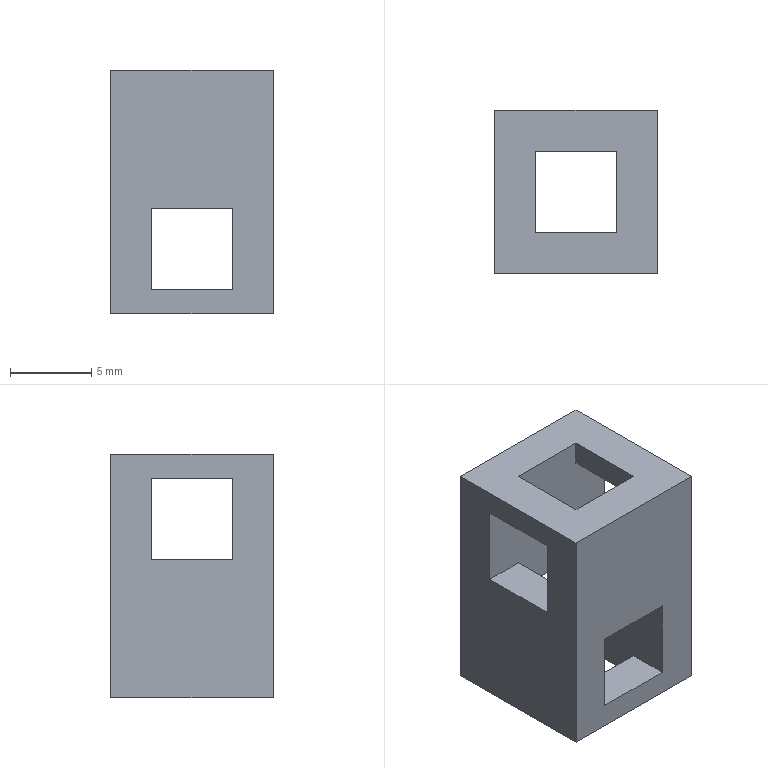Part | SolidWorks | features ICE 2, Extrusion 1 | 1 solid | 22 faces | box 10 x 10 x 15 mm | volume 875 mm3 | plane 22
STEP:
#1=CARTESIAN_POINT('',(2.5,2.5,8.5));
#2=VERTEX_POINT('',#1);
#3=CARTESIAN_POINT('',(2.5,-2.5,8.5));
#4=VERTEX_POINT('',#3);
#5=CARTESIAN_POINT('',(2.5,2.5,8.5));
#6=DIRECTION('',(0.,-1.,0.));
#7=VECTOR('',#6,1000.);
#8=LINE('',#5,#7);
#9=EDGE_CURVE('',#2,#4,#8,.T.);
#10=ORIENTED_EDGE('',*,*,#9,.F.);
#11=CARTESIAN_POINT('',(2.5,2.5,6.5));
#12=VERTEX_POINT('',#11);
#13=CARTESIAN_POINT('',(2.5,2.5,15.));
#14=DIRECTION('',(0.,0.,-1.));
#15=VECTOR('',#14,1000.);
#16=LINE('',#13,#15);
#17=EDGE_CURVE('',#2,#12,#16,.T.);
#18=ORIENTED_EDGE('',*,*,#17,.T.);
#19=CARTESIAN_POINT('',(2.5,5.,6.5));
#20=VERTEX_POINT('',#19);
#21=CARTESIAN_POINT('',(2.5,-5.,6.5));
#22=DIRECTION('',(0.,1.,0.));
#23=VECTOR('',#22,1000.);
#24=LINE('',#21,#23);
#25=EDGE_CURVE('',#12,#20,#24,.T.);
#26=ORIENTED_EDGE('',*,*,#25,.T.);
#27=CARTESIAN_POINT('',(2.5,5.,1.5));
#28=VERTEX_POINT('',#27);
#29=CARTESIAN_POINT('',(2.5,5.,1.5));
#30=DIRECTION('',(0.,0.,-1.));
#31=VECTOR('',#30,1000.);
#32=LINE('',#29,#31);
#33=EDGE_CURVE('',#20,#28,#32,.T.);
#34=ORIENTED_EDGE('',*,*,#33,.T.);
#35=CARTESIAN_POINT('',(2.5,2.5,1.5));
#36=VERTEX_POINT('',#35);
#37=CARTESIAN_POINT('',(2.5,-5.,1.5));
#38=DIRECTION('',(0.,1.,0.));
#39=VECTOR('',#38,1000.);
#40=LINE('',#37,#39);
#41=EDGE_CURVE('',#36,#28,#40,.T.);
#42=ORIENTED_EDGE('',*,*,#41,.F.);
#43=CARTESIAN_POINT('',(2.5,2.5,0.));
#44=VERTEX_POINT('',#43);
#45=CARTESIAN_POINT('',(2.5,2.5,15.));
#46=DIRECTION('',(0.,0.,-1.));
#47=VECTOR('',#46,1000.);
#48=LINE('',#45,#47);
#49=EDGE_CURVE('',#36,#44,#48,.T.);
#50=ORIENTED_EDGE('',*,*,#49,.T.);
#51=CARTESIAN_POINT('',(2.5,-2.5,0.));
#52=VERTEX_POINT('',#51);
#53=CARTESIAN_POINT('',(2.5,2.5,0.));
#54=DIRECTION('',(0.,1.,0.));
#55=VECTOR('',#54,1000.);
#56=LINE('',#53,#55);
#57=EDGE_CURVE('',#52,#44,#56,.T.);
#58=ORIENTED_EDGE('',*,*,#57,.F.);
#59=CARTESIAN_POINT('',(2.5,-2.5,1.5));
#60=VERTEX_POINT('',#59);
#61=CARTESIAN_POINT('',(2.5,-2.5,15.));
#62=DIRECTION('',(0.,0.,-1.));
#63=VECTOR('',#62,1000.);
#64=LINE('',#61,#63);
#65=EDGE_CURVE('',#60,#52,#64,.T.);
#66=ORIENTED_EDGE('',*,*,#65,.F.);
#67=CARTESIAN_POINT('',(2.5,-5.,1.5));
#68=VERTEX_POINT('',#67);
#69=CARTESIAN_POINT('',(2.5,-5.,1.5));
#70=DIRECTION('',(0.,1.,0.));
#71=VECTOR('',#70,1000.);
#72=LINE('',#69,#71);
#73=EDGE_CURVE('',#68,#60,#72,.T.);
#74=ORIENTED_EDGE('',*,*,#73,.F.);
#75=CARTESIAN_POINT('',(2.5,-5.,6.5));
#76=VERTEX_POINT('',#75);
#77=CARTESIAN_POINT('',(2.5,-5.,1.5));
#78=DIRECTION('',(0.,0.,-1.));
#79=VECTOR('',#78,1000.);
#80=LINE('',#77,#79);
#81=EDGE_CURVE('',#76,#68,#80,.T.);
#82=ORIENTED_EDGE('',*,*,#81,.F.);
#83=CARTESIAN_POINT('',(2.5,-2.5,6.5));
#84=VERTEX_POINT('',#83);
#85=CARTESIAN_POINT('',(2.5,-5.,6.5));
#86=DIRECTION('',(0.,1.,0.));
#87=VECTOR('',#86,1000.);
#88=LINE('',#85,#87);
#89=EDGE_CURVE('',#76,#84,#88,.T.);
#90=ORIENTED_EDGE('',*,*,#89,.T.);
#91=CARTESIAN_POINT('',(2.5,-2.5,15.));
#92=DIRECTION('',(0.,0.,-1.));
#93=VECTOR('',#92,1000.);
#94=LINE('',#91,#93);
#95=EDGE_CURVE('',#4,#84,#94,.T.);
#96=ORIENTED_EDGE('',*,*,#95,.F.);
#97=EDGE_LOOP('',(#10,#18,#26,#34,#42,#50,#58,#66,#74,#82,#90,#96));
#98=FACE_OUTER_BOUND('',#97,.T.);
#99=CARTESIAN_POINT('',(2.5,2.5,15.));
#100=DIRECTION('',(-1.,0.,0.));
#101=DIRECTION('',(0.,-1.,0.));
#102=AXIS2_PLACEMENT_3D('',#99,#100,#101);
#103=PLANE('',#102);
#104=ADVANCED_FACE('',(#98),#103,.T.);
#105=CARTESIAN_POINT('',(-2.5,-2.5,8.5));
#106=VERTEX_POINT('',#105);
#107=CARTESIAN_POINT('',(-2.5,2.5,8.5));
#108=VERTEX_POINT('',#107);
#109=CARTESIAN_POINT('',(-2.5,2.5,8.5));
#110=DIRECTION('',(0.,1.,0.));
#111=VECTOR('',#110,1000.);
#112=LINE('',#109,#111);
#113=EDGE_CURVE('',#106,#108,#112,.T.);
#114=ORIENTED_EDGE('',*,*,#113,.F.);
#115=CARTESIAN_POINT('',(-2.5,-2.5,6.5));
#116=VERTEX_POINT('',#115);
#117=CARTESIAN_POINT('',(-2.5,-2.5,15.));
#118=DIRECTION('',(0.,0.,-1.));
#119=VECTOR('',#118,1000.);
#120=LINE('',#117,#119);
#121=EDGE_CURVE('',#106,#116,#120,.T.);
#122=ORIENTED_EDGE('',*,*,#121,.T.);
#123=CARTESIAN_POINT('',(-2.5,-5.,6.5));
#124=VERTEX_POINT('',#123);
#125=CARTESIAN_POINT('',(-2.5,-5.,6.5));
#126=DIRECTION('',(0.,1.,0.));
#127=VECTOR('',#126,1000.);
#128=LINE('',#125,#127);
#129=EDGE_CURVE('',#124,#116,#128,.T.);
#130=ORIENTED_EDGE('',*,*,#129,.F.);
#131=CARTESIAN_POINT('',(-2.5,-5.,1.5));
#132=VERTEX_POINT('',#131);
#133=CARTESIAN_POINT('',(-2.5,-5.,1.5));
#134=DIRECTION('',(0.,0.,1.));
#135=VECTOR('',#134,1000.);
#136=LINE('',#133,#135);
#137=EDGE_CURVE('',#132,#124,#136,.T.);
#138=ORIENTED_EDGE('',*,*,#137,.F.);
#139=CARTESIAN_POINT('',(-2.5,-2.5,1.5));
#140=VERTEX_POINT('',#139);
#141=CARTESIAN_POINT('',(-2.5,-5.,1.5));
#142=DIRECTION('',(0.,1.,0.));
#143=VECTOR('',#142,1000.);
#144=LINE('',#141,#143);
#145=EDGE_CURVE('',#132,#140,#144,.T.);
#146=ORIENTED_EDGE('',*,*,#145,.T.);
#147=CARTESIAN_POINT('',(-2.5,-2.5,0.));
#148=VERTEX_POINT('',#147);
#149=CARTESIAN_POINT('',(-2.5,-2.5,15.));
#150=DIRECTION('',(0.,0.,-1.));
#151=VECTOR('',#150,1000.);
#152=LINE('',#149,#151);
#153=EDGE_CURVE('',#140,#148,#152,.T.);
#154=ORIENTED_EDGE('',*,*,#153,.T.);
#155=CARTESIAN_POINT('',(-2.5,2.5,0.));
#156=VERTEX_POINT('',#155);
#157=CARTESIAN_POINT('',(-2.5,2.5,0.));
#158=DIRECTION('',(0.,-1.,0.));
#159=VECTOR('',#158,1000.);
#160=LINE('',#157,#159);
#161=EDGE_CURVE('',#156,#148,#160,.T.);
#162=ORIENTED_EDGE('',*,*,#161,.F.);
#163=CARTESIAN_POINT('',(-2.5,2.5,1.5));
#164=VERTEX_POINT('',#163);
#165=CARTESIAN_POINT('',(-2.5,2.5,15.));
#166=DIRECTION('',(0.,0.,-1.));
#167=VECTOR('',#166,1000.);
#168=LINE('',#165,#167);
#169=EDGE_CURVE('',#164,#156,#168,.T.);
#170=ORIENTED_EDGE('',*,*,#169,.F.);
#171=CARTESIAN_POINT('',(-2.5,5.,1.5));
#172=VERTEX_POINT('',#171);
#173=CARTESIAN_POINT('',(-2.5,-5.,1.5));
#174=DIRECTION('',(0.,1.,0.));
#175=VECTOR('',#174,1000.);
#176=LINE('',#173,#175);
#177=EDGE_CURVE('',#164,#172,#176,.T.);
#178=ORIENTED_EDGE('',*,*,#177,.T.);
#179=CARTESIAN_POINT('',(-2.5,5.,6.5));
#180=VERTEX_POINT('',#179);
#181=CARTESIAN_POINT('',(-2.5,5.,1.5));
#182=DIRECTION('',(0.,0.,1.));
#183=VECTOR('',#182,1000.);
#184=LINE('',#181,#183);
#185=EDGE_CURVE('',#172,#180,#184,.T.);
#186=ORIENTED_EDGE('',*,*,#185,.T.);
#187=CARTESIAN_POINT('',(-2.5,2.5,6.5));
#188=VERTEX_POINT('',#187);
#189=CARTESIAN_POINT('',(-2.5,-5.,6.5));
#190=DIRECTION('',(0.,1.,0.));
#191=VECTOR('',#190,1000.);
#192=LINE('',#189,#191);
#193=EDGE_CURVE('',#188,#180,#192,.T.);
#194=ORIENTED_EDGE('',*,*,#193,.F.);
#195=CARTESIAN_POINT('',(-2.5,2.5,15.));
#196=DIRECTION('',(0.,0.,-1.));
#197=VECTOR('',#196,1000.);
#198=LINE('',#195,#197);
#199=EDGE_CURVE('',#108,#188,#198,.T.);
#200=ORIENTED_EDGE('',*,*,#199,.F.);
#201=EDGE_LOOP('',(#114,#122,#130,#138,#146,#154,#162,#170,#178,#186,#194,#200));
#202=FACE_OUTER_BOUND('',#201,.T.);
#203=CARTESIAN_POINT('',(-2.5,2.5,15.));
#204=DIRECTION('',(1.,0.,0.));
#205=DIRECTION('',(0.,1.,0.));
#206=AXIS2_PLACEMENT_3D('',#203,#204,#205);
#207=PLANE('',#206);
#208=ADVANCED_FACE('',(#202),#207,.T.);
#209=CARTESIAN_POINT('',(-2.5,2.5,15.));
#210=VERTEX_POINT('',#209);
#211=CARTESIAN_POINT('',(-2.5,2.5,13.5));
#212=VERTEX_POINT('',#211);
#213=CARTESIAN_POINT('',(-2.5,2.5,15.));
#214=DIRECTION('',(0.,0.,-1.));
#215=VECTOR('',#214,1000.);
#216=LINE('',#213,#215);
#217=EDGE_CURVE('',#210,#212,#216,.T.);
#218=ORIENTED_EDGE('',*,*,#217,.T.);
#219=CARTESIAN_POINT('',(-5.,2.5,13.5));
#220=VERTEX_POINT('',#219);
#221=CARTESIAN_POINT('',(-5.,2.5,13.5));
#222=DIRECTION('',(1.,0.,0.));
#223=VECTOR('',#222,1000.);
#224=LINE('',#221,#223);
#225=EDGE_CURVE('',#220,#212,#224,.T.);
#226=ORIENTED_EDGE('',*,*,#225,.F.);
#227=CARTESIAN_POINT('',(-5.,2.5,8.5));
#228=VERTEX_POINT('',#227);
#229=CARTESIAN_POINT('',(-5.,2.5,13.5));
#230=DIRECTION('',(0.,0.,1.));
#231=VECTOR('',#230,1000.);
#232=LINE('',#229,#231);
#233=EDGE_CURVE('',#228,#220,#232,.T.);
#234=ORIENTED_EDGE('',*,*,#233,.F.);
#235=CARTESIAN_POINT('',(-5.,2.5,8.5));
#236=DIRECTION('',(1.,0.,0.));
#237=VECTOR('',#236,1000.);
#238=LINE('',#235,#237);
#239=EDGE_CURVE('',#228,#108,#238,.T.);
#240=ORIENTED_EDGE('',*,*,#239,.T.);
#241=ORIENTED_EDGE('',*,*,#199,.T.);
#242=CARTESIAN_POINT('',(-2.5,2.5,6.5));
#243=DIRECTION('',(-1.,0.,0.));
#244=VECTOR('',#243,1000.);
#245=LINE('',#242,#244);
#246=EDGE_CURVE('',#12,#188,#245,.T.);
#247=ORIENTED_EDGE('',*,*,#246,.F.);
#248=ORIENTED_EDGE('',*,*,#17,.F.);
#249=CARTESIAN_POINT('',(5.,2.5,8.5));
#250=VERTEX_POINT('',#249);
#251=CARTESIAN_POINT('',(-5.,2.5,8.5));
#252=DIRECTION('',(1.,0.,0.));
#253=VECTOR('',#252,1000.);
#254=LINE('',#251,#253);
#255=EDGE_CURVE('',#2,#250,#254,.T.);
#256=ORIENTED_EDGE('',*,*,#255,.T.);
#257=CARTESIAN_POINT('',(5.,2.5,13.5));
#258=VERTEX_POINT('',#257);
#259=CARTESIAN_POINT('',(5.,2.5,13.5));
#260=DIRECTION('',(0.,0.,1.));
#261=VECTOR('',#260,1000.);
#262=LINE('',#259,#261);
#263=EDGE_CURVE('',#250,#258,#262,.T.);
#264=ORIENTED_EDGE('',*,*,#263,.T.);
#265=CARTESIAN_POINT('',(2.5,2.5,13.5));
#266=VERTEX_POINT('',#265);
#267=CARTESIAN_POINT('',(-5.,2.5,13.5));
#268=DIRECTION('',(1.,0.,0.));
#269=VECTOR('',#268,1000.);
#270=LINE('',#267,#269);
#271=EDGE_CURVE('',#266,#258,#270,.T.);
#272=ORIENTED_EDGE('',*,*,#271,.F.);
#273=CARTESIAN_POINT('',(2.5,2.5,15.));
#274=VERTEX_POINT('',#273);
#275=CARTESIAN_POINT('',(2.5,2.5,15.));
#276=DIRECTION('',(0.,0.,-1.));
#277=VECTOR('',#276,1000.);
#278=LINE('',#275,#277);
#279=EDGE_CURVE('',#274,#266,#278,.T.);
#280=ORIENTED_EDGE('',*,*,#279,.F.);
#281=CARTESIAN_POINT('',(-2.5,2.5,15.));
#282=DIRECTION('',(-1.,0.,0.));
#283=VECTOR('',#282,1000.);
#284=LINE('',#281,#283);
#285=EDGE_CURVE('',#274,#210,#284,.T.);
#286=ORIENTED_EDGE('',*,*,#285,.T.);
#287=EDGE_LOOP('',(#218,#226,#234,#240,#241,#247,#248,#256,#264,#272,#280,#286));
#288=FACE_OUTER_BOUND('',#287,.T.);
#289=CARTESIAN_POINT('',(-2.5,2.5,15.));
#290=DIRECTION('',(0.,-1.,0.));
#291=DIRECTION('',(0.,0.,-1.));
#292=AXIS2_PLACEMENT_3D('',#289,#290,#291);
#293=PLANE('',#292);
#294=ADVANCED_FACE('',(#288),#293,.T.);
#295=CARTESIAN_POINT('',(2.5,-2.5,15.));
#296=VERTEX_POINT('',#295);
#297=CARTESIAN_POINT('',(2.5,-2.5,13.5));
#298=VERTEX_POINT('',#297);
#299=CARTESIAN_POINT('',(2.5,-2.5,15.));
#300=DIRECTION('',(0.,0.,-1.));
#301=VECTOR('',#300,1000.);
#302=LINE('',#299,#301);
#303=EDGE_CURVE('',#296,#298,#302,.T.);
#304=ORIENTED_EDGE('',*,*,#303,.T.);
#305=CARTESIAN_POINT('',(5.,-2.5,13.5));
#306=VERTEX_POINT('',#305);
#307=CARTESIAN_POINT('',(-5.,-2.5,13.5));
#308=DIRECTION('',(1.,0.,0.));
#309=VECTOR('',#308,1000.);
#310=LINE('',#307,#309);
#311=EDGE_CURVE('',#298,#306,#310,.T.);
#312=ORIENTED_EDGE('',*,*,#311,.T.);
#313=CARTESIAN_POINT('',(5.,-2.5,8.5));
#314=VERTEX_POINT('',#313);
#315=CARTESIAN_POINT('',(5.,-2.5,13.5));
#316=DIRECTION('',(0.,0.,-1.));
#317=VECTOR('',#316,1000.);
#318=LINE('',#315,#317);
#319=EDGE_CURVE('',#306,#314,#318,.T.);
#320=ORIENTED_EDGE('',*,*,#319,.T.);
#321=CARTESIAN_POINT('',(-5.,-2.5,8.5));
#322=DIRECTION('',(1.,0.,0.));
#323=VECTOR('',#322,1000.);
#324=LINE('',#321,#323);
#325=EDGE_CURVE('',#4,#314,#324,.T.);
#326=ORIENTED_EDGE('',*,*,#325,.F.);
#327=ORIENTED_EDGE('',*,*,#95,.T.);
#328=CARTESIAN_POINT('',(-2.5,-2.5,6.5));
#329=DIRECTION('',(1.,0.,0.));
#330=VECTOR('',#329,1000.);
#331=LINE('',#328,#330);
#332=EDGE_CURVE('',#116,#84,#331,.T.);
#333=ORIENTED_EDGE('',*,*,#332,.F.);
#334=ORIENTED_EDGE('',*,*,#121,.F.);
#335=CARTESIAN_POINT('',(-5.,-2.5,8.5));
#336=VERTEX_POINT('',#335);
#337=CARTESIAN_POINT('',(-5.,-2.5,8.5));
#338=DIRECTION('',(1.,0.,0.));
#339=VECTOR('',#338,1000.);
#340=LINE('',#337,#339);
#341=EDGE_CURVE('',#336,#106,#340,.T.);
#342=ORIENTED_EDGE('',*,*,#341,.F.);
#343=CARTESIAN_POINT('',(-5.,-2.5,13.5));
#344=VERTEX_POINT('',#343);
#345=CARTESIAN_POINT('',(-5.,-2.5,13.5));
#346=DIRECTION('',(0.,0.,-1.));
#347=VECTOR('',#346,1000.);
#348=LINE('',#345,#347);
#349=EDGE_CURVE('',#344,#336,#348,.T.);
#350=ORIENTED_EDGE('',*,*,#349,.F.);
#351=CARTESIAN_POINT('',(-2.5,-2.5,13.5));
#352=VERTEX_POINT('',#351);
#353=CARTESIAN_POINT('',(-5.,-2.5,13.5));
#354=DIRECTION('',(1.,0.,0.));
#355=VECTOR('',#354,1000.);
#356=LINE('',#353,#355);
#357=EDGE_CURVE('',#344,#352,#356,.T.);
#358=ORIENTED_EDGE('',*,*,#357,.T.);
#359=CARTESIAN_POINT('',(-2.5,-2.5,15.));
#360=VERTEX_POINT('',#359);
#361=CARTESIAN_POINT('',(-2.5,-2.5,15.));
#362=DIRECTION('',(0.,0.,-1.));
#363=VECTOR('',#362,1000.);
#364=LINE('',#361,#363);
#365=EDGE_CURVE('',#360,#352,#364,.T.);
#366=ORIENTED_EDGE('',*,*,#365,.F.);
#367=CARTESIAN_POINT('',(-2.5,-2.5,15.));
#368=DIRECTION('',(1.,0.,0.));
#369=VECTOR('',#368,1000.);
#370=LINE('',#367,#369);
#371=EDGE_CURVE('',#360,#296,#370,.T.);
#372=ORIENTED_EDGE('',*,*,#371,.T.);
#373=EDGE_LOOP('',(#304,#312,#320,#326,#327,#333,#334,#342,#350,#358,#366,#372));
#374=FACE_OUTER_BOUND('',#373,.T.);
#375=CARTESIAN_POINT('',(-2.5,-2.5,15.));
#376=DIRECTION('',(0.,1.,0.));
#377=DIRECTION('',(0.,0.,1.));
#378=AXIS2_PLACEMENT_3D('',#375,#376,#377);
#379=PLANE('',#378);
#380=ADVANCED_FACE('',(#374),#379,.T.);
#381=CARTESIAN_POINT('',(5.,-5.,15.));
#382=VERTEX_POINT('',#381);
#383=CARTESIAN_POINT('',(5.,5.,15.));
#384=VERTEX_POINT('',#383);
#385=CARTESIAN_POINT('',(5.,5.,15.));
#386=DIRECTION('',(0.,1.,0.));
#387=VECTOR('',#386,1000.);
#388=LINE('',#385,#387);
#389=EDGE_CURVE('',#382,#384,#388,.T.);
#390=ORIENTED_EDGE('',*,*,#389,.T.);
#391=CARTESIAN_POINT('',(-5.,5.,15.));
#392=VERTEX_POINT('',#391);
#393=CARTESIAN_POINT('',(-5.,5.,15.));
#394=DIRECTION('',(-1.,0.,0.));
#395=VECTOR('',#394,1000.);
#396=LINE('',#393,#395);
#397=EDGE_CURVE('',#384,#392,#396,.T.);
#398=ORIENTED_EDGE('',*,*,#397,.T.);
#399=CARTESIAN_POINT('',(-5.,-5.,15.));
#400=VERTEX_POINT('',#399);
#401=CARTESIAN_POINT('',(-5.,5.,15.));
#402=DIRECTION('',(0.,-1.,0.));
#403=VECTOR('',#402,1000.);
#404=LINE('',#401,#403);
#405=EDGE_CURVE('',#392,#400,#404,.T.);
#406=ORIENTED_EDGE('',*,*,#405,.T.);
#407=CARTESIAN_POINT('',(-5.,-5.,15.));
#408=DIRECTION('',(1.,0.,0.));
#409=VECTOR('',#408,1000.);
#410=LINE('',#407,#409);
#411=EDGE_CURVE('',#400,#382,#410,.T.);
#412=ORIENTED_EDGE('',*,*,#411,.T.);
#413=EDGE_LOOP('',(#390,#398,#406,#412));
#414=FACE_OUTER_BOUND('',#413,.T.);
#415=ORIENTED_EDGE('',*,*,#285,.F.);
#416=CARTESIAN_POINT('',(2.5,2.5,15.));
#417=DIRECTION('',(0.,1.,0.));
#418=VECTOR('',#417,1000.);
#419=LINE('',#416,#418);
#420=EDGE_CURVE('',#296,#274,#419,.T.);
#421=ORIENTED_EDGE('',*,*,#420,.F.);
#422=ORIENTED_EDGE('',*,*,#371,.F.);
#423=CARTESIAN_POINT('',(-2.5,2.5,15.));
#424=DIRECTION('',(0.,-1.,0.));
#425=VECTOR('',#424,1000.);
#426=LINE('',#423,#425);
#427=EDGE_CURVE('',#210,#360,#426,.T.);
#428=ORIENTED_EDGE('',*,*,#427,.F.);
#429=EDGE_LOOP('',(#415,#421,#422,#428));
#430=FACE_BOUND('',#429,.T.);
#431=CARTESIAN_POINT('',(0.,0.,15.));
#432=DIRECTION('',(0.,0.,1.));
#433=DIRECTION('',(1.,0.,0.));
#434=AXIS2_PLACEMENT_3D('',#431,#432,#433);
#435=PLANE('',#434);
#436=ADVANCED_FACE('',(#414,#430),#435,.T.);
#437=CARTESIAN_POINT('',(5.,-5.,0.));
#438=VERTEX_POINT('',#437);
#439=CARTESIAN_POINT('',(5.,5.,0.));
#440=VERTEX_POINT('',#439);
#441=CARTESIAN_POINT('',(5.,5.,0.));
#442=DIRECTION('',(0.,1.,0.));
#443=VECTOR('',#442,1000.);
#444=LINE('',#441,#443);
#445=EDGE_CURVE('',#438,#440,#444,.T.);
#446=ORIENTED_EDGE('',*,*,#445,.F.);
#447=CARTESIAN_POINT('',(-5.,-5.,0.));
#448=VERTEX_POINT('',#447);
#449=CARTESIAN_POINT('',(-5.,-5.,0.));
#450=DIRECTION('',(1.,0.,0.));
#451=VECTOR('',#450,1000.);
#452=LINE('',#449,#451);
#453=EDGE_CURVE('',#448,#438,#452,.T.);
#454=ORIENTED_EDGE('',*,*,#453,.F.);
#455=CARTESIAN_POINT('',(-5.,5.,0.));
#456=VERTEX_POINT('',#455);
#457=CARTESIAN_POINT('',(-5.,5.,0.));
#458=DIRECTION('',(0.,-1.,0.));
#459=VECTOR('',#458,1000.);
#460=LINE('',#457,#459);
#461=EDGE_CURVE('',#456,#448,#460,.T.);
#462=ORIENTED_EDGE('',*,*,#461,.F.);
#463=CARTESIAN_POINT('',(-5.,5.,0.));
#464=DIRECTION('',(-1.,0.,0.));
#465=VECTOR('',#464,1000.);
#466=LINE('',#463,#465);
#467=EDGE_CURVE('',#440,#456,#466,.T.);
#468=ORIENTED_EDGE('',*,*,#467,.F.);
#469=EDGE_LOOP('',(#446,#454,#462,#468));
#470=FACE_OUTER_BOUND('',#469,.T.);
#471=ORIENTED_EDGE('',*,*,#57,.T.);
#472=CARTESIAN_POINT('',(-2.5,2.5,0.));
#473=DIRECTION('',(-1.,0.,0.));
#474=VECTOR('',#473,1000.);
#475=LINE('',#472,#474);
#476=EDGE_CURVE('',#44,#156,#475,.T.);
#477=ORIENTED_EDGE('',*,*,#476,.T.);
#478=ORIENTED_EDGE('',*,*,#161,.T.);
#479=CARTESIAN_POINT('',(-2.5,-2.5,0.));
#480=DIRECTION('',(1.,0.,0.));
#481=VECTOR('',#480,1000.);
#482=LINE('',#479,#481);
#483=EDGE_CURVE('',#148,#52,#482,.T.);
#484=ORIENTED_EDGE('',*,*,#483,.T.);
#485=EDGE_LOOP('',(#471,#477,#478,#484));
#486=FACE_BOUND('',#485,.T.);
#487=CARTESIAN_POINT('',(0.,0.,0.));
#488=DIRECTION('',(0.,0.,1.));
#489=DIRECTION('',(1.,0.,0.));
#490=AXIS2_PLACEMENT_3D('',#487,#488,#489);
#491=PLANE('',#490);
#492=ADVANCED_FACE('',(#470,#486),#491,.F.);
#493=ORIENTED_EDGE('',*,*,#263,.F.);
#494=CARTESIAN_POINT('',(5.,2.5,8.5));
#495=DIRECTION('',(0.,1.,0.));
#496=VECTOR('',#495,1000.);
#497=LINE('',#494,#496);
#498=EDGE_CURVE('',#314,#250,#497,.T.);
#499=ORIENTED_EDGE('',*,*,#498,.F.);
#500=ORIENTED_EDGE('',*,*,#319,.F.);
#501=CARTESIAN_POINT('',(5.,2.5,13.5));
#502=DIRECTION('',(0.,-1.,0.));
#503=VECTOR('',#502,1000.);
#504=LINE('',#501,#503);
#505=EDGE_CURVE('',#258,#306,#504,.T.);
#506=ORIENTED_EDGE('',*,*,#505,.F.);
#507=EDGE_LOOP('',(#493,#499,#500,#506));
#508=FACE_BOUND('',#507,.T.);
#509=ORIENTED_EDGE('',*,*,#445,.T.);
#510=CARTESIAN_POINT('',(5.,5.,15.));
#511=DIRECTION('',(0.,0.,-1.));
#512=VECTOR('',#511,1000.);
#513=LINE('',#510,#512);
#514=EDGE_CURVE('',#384,#440,#513,.T.);
#515=ORIENTED_EDGE('',*,*,#514,.F.);
#516=ORIENTED_EDGE('',*,*,#389,.F.);
#517=CARTESIAN_POINT('',(5.,-5.,15.));
#518=DIRECTION('',(0.,0.,-1.));
#519=VECTOR('',#518,1000.);
#520=LINE('',#517,#519);
#521=EDGE_CURVE('',#382,#438,#520,.T.);
#522=ORIENTED_EDGE('',*,*,#521,.T.);
#523=EDGE_LOOP('',(#509,#515,#516,#522));
#524=FACE_OUTER_BOUND('',#523,.T.);
#525=CARTESIAN_POINT('',(5.,5.,15.));
#526=DIRECTION('',(-1.,0.,0.));
#527=DIRECTION('',(0.,-1.,0.));
#528=AXIS2_PLACEMENT_3D('',#525,#526,#527);
#529=PLANE('',#528);
#530=ADVANCED_FACE('',(#508,#524),#529,.F.);
#531=CARTESIAN_POINT('',(-2.5,5.,1.5));
#532=DIRECTION('',(-1.,0.,0.));
#533=VECTOR('',#532,1000.);
#534=LINE('',#531,#533);
#535=EDGE_CURVE('',#28,#172,#534,.T.);
#536=ORIENTED_EDGE('',*,*,#535,.F.);
#537=ORIENTED_EDGE('',*,*,#33,.F.);
#538=CARTESIAN_POINT('',(-2.5,5.,6.5));
#539=DIRECTION('',(1.,0.,0.));
#540=VECTOR('',#539,1000.);
#541=LINE('',#538,#540);
#542=EDGE_CURVE('',#180,#20,#541,.T.);
#543=ORIENTED_EDGE('',*,*,#542,.F.);
#544=ORIENTED_EDGE('',*,*,#185,.F.);
#545=EDGE_LOOP('',(#536,#537,#543,#544));
#546=FACE_BOUND('',#545,.T.);
#547=ORIENTED_EDGE('',*,*,#467,.T.);
#548=CARTESIAN_POINT('',(-5.,5.,15.));
#549=DIRECTION('',(0.,0.,-1.));
#550=VECTOR('',#549,1000.);
#551=LINE('',#548,#550);
#552=EDGE_CURVE('',#392,#456,#551,.T.);
#553=ORIENTED_EDGE('',*,*,#552,.F.);
#554=ORIENTED_EDGE('',*,*,#397,.F.);
#555=ORIENTED_EDGE('',*,*,#514,.T.);
#556=EDGE_LOOP('',(#547,#553,#554,#555));
#557=FACE_OUTER_BOUND('',#556,.T.);
#558=CARTESIAN_POINT('',(-5.,5.,15.));
#559=DIRECTION('',(0.,-1.,0.));
#560=DIRECTION('',(0.,0.,-1.));
#561=AXIS2_PLACEMENT_3D('',#558,#559,#560);
#562=PLANE('',#561);
#563=ADVANCED_FACE('',(#546,#557),#562,.F.);
#564=ORIENTED_EDGE('',*,*,#349,.T.);
#565=CARTESIAN_POINT('',(-5.,2.5,8.5));
#566=DIRECTION('',(0.,1.,0.));
#567=VECTOR('',#566,1000.);
#568=LINE('',#565,#567);
#569=EDGE_CURVE('',#336,#228,#568,.T.);
#570=ORIENTED_EDGE('',*,*,#569,.T.);
#571=ORIENTED_EDGE('',*,*,#233,.T.);
#572=CARTESIAN_POINT('',(-5.,2.5,13.5));
#573=DIRECTION('',(0.,-1.,0.));
#574=VECTOR('',#573,1000.);
#575=LINE('',#572,#574);
#576=EDGE_CURVE('',#220,#344,#575,.T.);
#577=ORIENTED_EDGE('',*,*,#576,.T.);
#578=EDGE_LOOP('',(#564,#570,#571,#577));
#579=FACE_BOUND('',#578,.T.);
#580=ORIENTED_EDGE('',*,*,#461,.T.);
#581=CARTESIAN_POINT('',(-5.,-5.,15.));
#582=DIRECTION('',(0.,0.,-1.));
#583=VECTOR('',#582,1000.);
#584=LINE('',#581,#583);
#585=EDGE_CURVE('',#400,#448,#584,.T.);
#586=ORIENTED_EDGE('',*,*,#585,.F.);
#587=ORIENTED_EDGE('',*,*,#405,.F.);
#588=ORIENTED_EDGE('',*,*,#552,.T.);
#589=EDGE_LOOP('',(#580,#586,#587,#588));
#590=FACE_OUTER_BOUND('',#589,.T.);
#591=CARTESIAN_POINT('',(-5.,5.,15.));
#592=DIRECTION('',(1.,0.,0.));
#593=DIRECTION('',(0.,1.,0.));
#594=AXIS2_PLACEMENT_3D('',#591,#592,#593);
#595=PLANE('',#594);
#596=ADVANCED_FACE('',(#579,#590),#595,.F.);
#597=CARTESIAN_POINT('',(-2.5,-5.,6.5));
#598=DIRECTION('',(1.,0.,0.));
#599=VECTOR('',#598,1000.);
#600=LINE('',#597,#599);
#601=EDGE_CURVE('',#124,#76,#600,.T.);
#602=ORIENTED_EDGE('',*,*,#601,.T.);
#603=ORIENTED_EDGE('',*,*,#81,.T.);
#604=CARTESIAN_POINT('',(-2.5,-5.,1.5));
#605=DIRECTION('',(-1.,0.,0.));
#606=VECTOR('',#605,1000.);
#607=LINE('',#604,#606);
#608=EDGE_CURVE('',#68,#132,#607,.T.);
#609=ORIENTED_EDGE('',*,*,#608,.T.);
#610=ORIENTED_EDGE('',*,*,#137,.T.);
#611=EDGE_LOOP('',(#602,#603,#609,#610));
#612=FACE_BOUND('',#611,.T.);
#613=ORIENTED_EDGE('',*,*,#453,.T.);
#614=ORIENTED_EDGE('',*,*,#521,.F.);
#615=ORIENTED_EDGE('',*,*,#411,.F.);
#616=ORIENTED_EDGE('',*,*,#585,.T.);
#617=EDGE_LOOP('',(#613,#614,#615,#616));
#618=FACE_OUTER_BOUND('',#617,.T.);
#619=CARTESIAN_POINT('',(-5.,-5.,15.));
#620=DIRECTION('',(0.,1.,0.));
#621=DIRECTION('',(0.,0.,1.));
#622=AXIS2_PLACEMENT_3D('',#619,#620,#621);
#623=PLANE('',#622);
#624=ADVANCED_FACE('',(#612,#618),#623,.F.);
#625=CARTESIAN_POINT('',(2.5,2.5,13.5));
#626=DIRECTION('',(0.,1.,0.));
#627=VECTOR('',#626,1000.);
#628=LINE('',#625,#627);
#629=EDGE_CURVE('',#298,#266,#628,.T.);
#630=ORIENTED_EDGE('',*,*,#629,.F.);
#631=ORIENTED_EDGE('',*,*,#303,.F.);
#632=ORIENTED_EDGE('',*,*,#420,.T.);
#633=ORIENTED_EDGE('',*,*,#279,.T.);
#634=EDGE_LOOP('',(#630,#631,#632,#633));
#635=FACE_OUTER_BOUND('',#634,.T.);
#636=CARTESIAN_POINT('',(2.5,2.5,15.));
#637=DIRECTION('',(-1.,0.,0.));
#638=DIRECTION('',(0.,-1.,0.));
#639=AXIS2_PLACEMENT_3D('',#636,#637,#638);
#640=PLANE('',#639);
#641=ADVANCED_FACE('',(#635),#640,.T.);
#642=CARTESIAN_POINT('',(-2.5,2.5,1.5));
#643=DIRECTION('',(1.,0.,0.));
#644=VECTOR('',#643,1000.);
#645=LINE('',#642,#644);
#646=EDGE_CURVE('',#164,#36,#645,.T.);
#647=ORIENTED_EDGE('',*,*,#646,.F.);
#648=ORIENTED_EDGE('',*,*,#169,.T.);
#649=ORIENTED_EDGE('',*,*,#476,.F.);
#650=ORIENTED_EDGE('',*,*,#49,.F.);
#651=EDGE_LOOP('',(#647,#648,#649,#650));
#652=FACE_OUTER_BOUND('',#651,.T.);
#653=CARTESIAN_POINT('',(-2.5,2.5,15.));
#654=DIRECTION('',(0.,-1.,0.));
#655=DIRECTION('',(0.,0.,-1.));
#656=AXIS2_PLACEMENT_3D('',#653,#654,#655);
#657=PLANE('',#656);
#658=ADVANCED_FACE('',(#652),#657,.T.);
#659=CARTESIAN_POINT('',(-2.5,2.5,13.5));
#660=DIRECTION('',(0.,-1.,0.));
#661=VECTOR('',#660,1000.);
#662=LINE('',#659,#661);
#663=EDGE_CURVE('',#212,#352,#662,.T.);
#664=ORIENTED_EDGE('',*,*,#663,.F.);
#665=ORIENTED_EDGE('',*,*,#217,.F.);
#666=ORIENTED_EDGE('',*,*,#427,.T.);
#667=ORIENTED_EDGE('',*,*,#365,.T.);
#668=EDGE_LOOP('',(#664,#665,#666,#667));
#669=FACE_OUTER_BOUND('',#668,.T.);
#670=CARTESIAN_POINT('',(-2.5,2.5,15.));
#671=DIRECTION('',(1.,0.,0.));
#672=DIRECTION('',(0.,1.,0.));
#673=AXIS2_PLACEMENT_3D('',#670,#671,#672);
#674=PLANE('',#673);
#675=ADVANCED_FACE('',(#669),#674,.T.);
#676=CARTESIAN_POINT('',(-2.5,-2.5,1.5));
#677=DIRECTION('',(-1.,0.,0.));
#678=VECTOR('',#677,1000.);
#679=LINE('',#676,#678);
#680=EDGE_CURVE('',#60,#140,#679,.T.);
#681=ORIENTED_EDGE('',*,*,#680,.F.);
#682=ORIENTED_EDGE('',*,*,#65,.T.);
#683=ORIENTED_EDGE('',*,*,#483,.F.);
#684=ORIENTED_EDGE('',*,*,#153,.F.);
#685=EDGE_LOOP('',(#681,#682,#683,#684));
#686=FACE_OUTER_BOUND('',#685,.T.);
#687=CARTESIAN_POINT('',(-2.5,-2.5,15.));
#688=DIRECTION('',(0.,1.,0.));
#689=DIRECTION('',(0.,0.,1.));
#690=AXIS2_PLACEMENT_3D('',#687,#688,#689);
#691=PLANE('',#690);
#692=ADVANCED_FACE('',(#686),#691,.T.);
#693=ORIENTED_EDGE('',*,*,#680,.T.);
#694=ORIENTED_EDGE('',*,*,#145,.F.);
#695=ORIENTED_EDGE('',*,*,#608,.F.);
#696=ORIENTED_EDGE('',*,*,#73,.T.);
#697=EDGE_LOOP('',(#693,#694,#695,#696));
#698=FACE_OUTER_BOUND('',#697,.T.);
#699=CARTESIAN_POINT('',(-2.5,-5.,1.5));
#700=DIRECTION('',(0.,0.,-1.));
#701=DIRECTION('',(-1.,0.,0.));
#702=AXIS2_PLACEMENT_3D('',#699,#700,#701);
#703=PLANE('',#702);
#704=ADVANCED_FACE('',(#698),#703,.F.);
#705=ORIENTED_EDGE('',*,*,#332,.T.);
#706=ORIENTED_EDGE('',*,*,#89,.F.);
#707=ORIENTED_EDGE('',*,*,#601,.F.);
#708=ORIENTED_EDGE('',*,*,#129,.T.);
#709=EDGE_LOOP('',(#705,#706,#707,#708));
#710=FACE_OUTER_BOUND('',#709,.T.);
#711=CARTESIAN_POINT('',(-2.5,-5.,6.5));
#712=DIRECTION('',(0.,0.,1.));
#713=DIRECTION('',(1.,0.,0.));
#714=AXIS2_PLACEMENT_3D('',#711,#712,#713);
#715=PLANE('',#714);
#716=ADVANCED_FACE('',(#710),#715,.F.);
#717=ORIENTED_EDGE('',*,*,#246,.T.);
#718=ORIENTED_EDGE('',*,*,#193,.T.);
#719=ORIENTED_EDGE('',*,*,#542,.T.);
#720=ORIENTED_EDGE('',*,*,#25,.F.);
#721=EDGE_LOOP('',(#717,#718,#719,#720));
#722=FACE_OUTER_BOUND('',#721,.T.);
#723=CARTESIAN_POINT('',(-2.5,-5.,6.5));
#724=DIRECTION('',(0.,0.,1.));
#725=DIRECTION('',(1.,0.,0.));
#726=AXIS2_PLACEMENT_3D('',#723,#724,#725);
#727=PLANE('',#726);
#728=ADVANCED_FACE('',(#722),#727,.F.);
#729=ORIENTED_EDGE('',*,*,#646,.T.);
#730=ORIENTED_EDGE('',*,*,#41,.T.);
#731=ORIENTED_EDGE('',*,*,#535,.T.);
#732=ORIENTED_EDGE('',*,*,#177,.F.);
#733=EDGE_LOOP('',(#729,#730,#731,#732));
#734=FACE_OUTER_BOUND('',#733,.T.);
#735=CARTESIAN_POINT('',(-2.5,-5.,1.5));
#736=DIRECTION('',(0.,0.,-1.));
#737=DIRECTION('',(-1.,0.,0.));
#738=AXIS2_PLACEMENT_3D('',#735,#736,#737);
#739=PLANE('',#738);
#740=ADVANCED_FACE('',(#734),#739,.F.);
#741=ORIENTED_EDGE('',*,*,#663,.T.);
#742=ORIENTED_EDGE('',*,*,#357,.F.);
#743=ORIENTED_EDGE('',*,*,#576,.F.);
#744=ORIENTED_EDGE('',*,*,#225,.T.);
#745=EDGE_LOOP('',(#741,#742,#743,#744));
#746=FACE_OUTER_BOUND('',#745,.T.);
#747=CARTESIAN_POINT('',(-5.,2.5,13.5));
#748=DIRECTION('',(0.,0.,1.));
#749=DIRECTION('',(1.,0.,0.));
#750=AXIS2_PLACEMENT_3D('',#747,#748,#749);
#751=PLANE('',#750);
#752=ADVANCED_FACE('',(#746),#751,.F.);
#753=ORIENTED_EDGE('',*,*,#113,.T.);
#754=ORIENTED_EDGE('',*,*,#239,.F.);
#755=ORIENTED_EDGE('',*,*,#569,.F.);
#756=ORIENTED_EDGE('',*,*,#341,.T.);
#757=EDGE_LOOP('',(#753,#754,#755,#756));
#758=FACE_OUTER_BOUND('',#757,.T.);
#759=CARTESIAN_POINT('',(-5.,2.5,8.5));
#760=DIRECTION('',(0.,0.,-1.));
#761=DIRECTION('',(-1.,0.,0.));
#762=AXIS2_PLACEMENT_3D('',#759,#760,#761);
#763=PLANE('',#762);
#764=ADVANCED_FACE('',(#758),#763,.F.);
#765=ORIENTED_EDGE('',*,*,#9,.T.);
#766=ORIENTED_EDGE('',*,*,#325,.T.);
#767=ORIENTED_EDGE('',*,*,#498,.T.);
#768=ORIENTED_EDGE('',*,*,#255,.F.);
#769=EDGE_LOOP('',(#765,#766,#767,#768));
#770=FACE_OUTER_BOUND('',#769,.T.);
#771=CARTESIAN_POINT('',(-5.,2.5,8.5));
#772=DIRECTION('',(0.,0.,-1.));
#773=DIRECTION('',(-1.,0.,0.));
#774=AXIS2_PLACEMENT_3D('',#771,#772,#773);
#775=PLANE('',#774);
#776=ADVANCED_FACE('',(#770),#775,.F.);
#777=ORIENTED_EDGE('',*,*,#629,.T.);
#778=ORIENTED_EDGE('',*,*,#271,.T.);
#779=ORIENTED_EDGE('',*,*,#505,.T.);
#780=ORIENTED_EDGE('',*,*,#311,.F.);
#781=EDGE_LOOP('',(#777,#778,#779,#780));
#782=FACE_OUTER_BOUND('',#781,.T.);
#783=CARTESIAN_POINT('',(-5.,2.5,13.5));
#784=DIRECTION('',(0.,0.,1.));
#785=DIRECTION('',(1.,0.,0.));
#786=AXIS2_PLACEMENT_3D('',#783,#784,#785);
#787=PLANE('',#786);
#788=ADVANCED_FACE('',(#782),#787,.F.);
#789=CLOSED_SHELL('',(#104,#208,#294,#380,#436,#492,#530,#563,#596,#624,#641,#658,#675,#692,#704,#716,#728,#740,#752,#764,#776,#788));
#790=MANIFOLD_SOLID_BREP('',#789);
#791=CARTESIAN_POINT('',(0.,0.,0.));
#792=DIRECTION('',(0.,0.,1.));
#793=DIRECTION('',(1.,0.,0.));
#794=AXIS2_PLACEMENT_3D('',#791,#792,#793);
#795=(LENGTH_UNIT()NAMED_UNIT(*)SI_UNIT(.MILLI.,.METRE.));
#796=UNCERTAINTY_MEASURE_WITH_UNIT(LENGTH_MEASURE(0.00001),#795,'','');
#797=(NAMED_UNIT(*)PLANE_ANGLE_UNIT()SI_UNIT($,.RADIAN.));
#798=(NAMED_UNIT(*)SI_UNIT($,.STERADIAN.)SOLID_ANGLE_UNIT());
#799=(GEOMETRIC_REPRESENTATION_CONTEXT(3)GLOBAL_UNCERTAINTY_ASSIGNED_CONTEXT((#796))GLOBAL_UNIT_ASSIGNED_CONTEXT((#795,#797,#798))REPRESENTATION_CONTEXT('',''));
#800=ADVANCED_BREP_SHAPE_REPRESENTATION('',(#790,#794),#799);